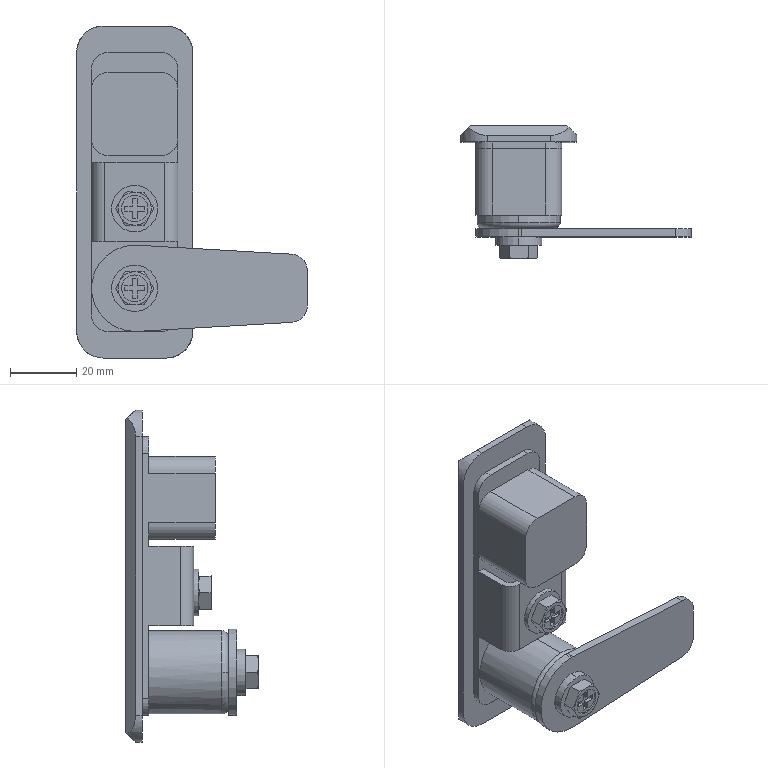Part | SolidWorks | features BaseBody 1 | 1 solid | 163 faces | box 69.5 x 40 x 100 mm | volume 51575 mm3 | plane 92 | cylinder 45 | cone 24 | torus 2 | commonest cylinder face diameters 10 x10 4 x6 8 x6 14 x4 16 x4 20.6 x3